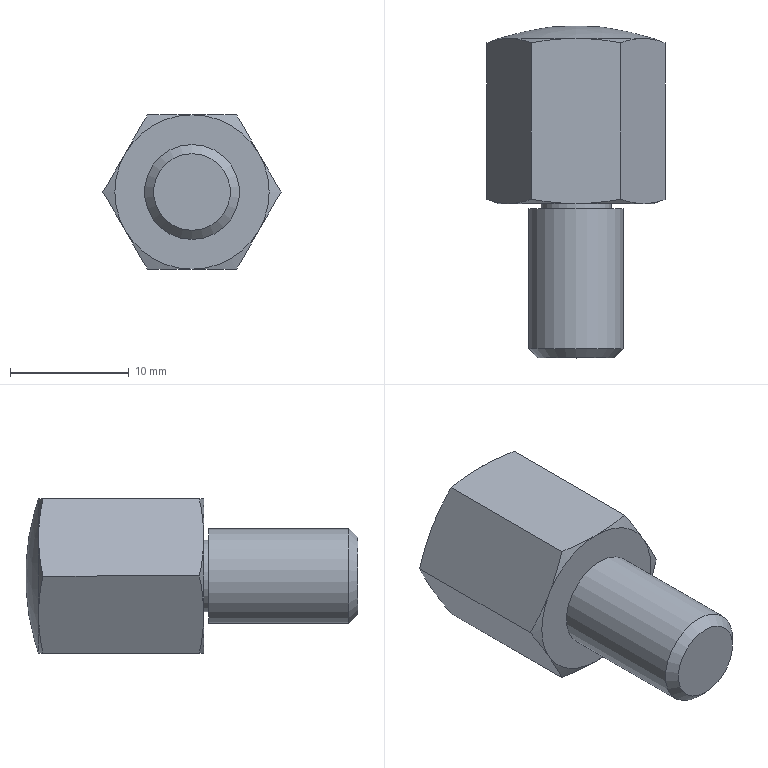Part | NX | features BREP 1 | 1 solid | 25 faces | box 15.011 x 28 x 13 mm | volume 2743 mm3 | cone 13 | plane 9 | cylinder 2 | sphere 1 | commonest cylinder face diameters 6 x1 8 x1
STEP:
#1=CARTESIAN_POINT('',(0.,-0.4333,4.));
#2=VERTEX_POINT('',#1);
#3=CARTESIAN_POINT('',(0.,-0.4333,0.));
#4=DIRECTION('',(0.,-1.,0.));
#5=DIRECTION('',(0.,0.,1.));
#6=AXIS2_PLACEMENT_3D('',#3,#4,#5);
#7=CIRCLE('',#6,4.);
#8=EDGE_CURVE('',#2,#2,#7,.T.);
#9=ORIENTED_EDGE('',*,*,#8,.T.);
#10=EDGE_LOOP('',(#9));
#11=FACE_BOUND('',#10,.T.);
#12=CARTESIAN_POINT('',(0.,-12.233,4.));
#13=VERTEX_POINT('',#12);
#14=CARTESIAN_POINT('',(0.,-12.233,0.));
#15=DIRECTION('',(0.,1.,0.));
#16=DIRECTION('',(0.,0.,1.));
#17=AXIS2_PLACEMENT_3D('',#14,#15,#16);
#18=CIRCLE('',#17,4.);
#19=EDGE_CURVE('',#13,#13,#18,.T.);
#20=ORIENTED_EDGE('',*,*,#19,.T.);
#21=EDGE_LOOP('',(#20));
#22=FACE_BOUND('',#21,.T.);
#23=CARTESIAN_POINT('',(0.,-6.333,0.));
#24=DIRECTION('',(0.,1.,0.));
#25=DIRECTION('',(0.,0.,-1.));
#26=AXIS2_PLACEMENT_3D('',#23,#24,#25);
#27=CYLINDRICAL_SURFACE('',#26,4.);
#28=ADVANCED_FACE('',(#11,#22),#27,.T.);
#29=ORIENTED_EDGE('',*,*,#8,.F.);
#30=EDGE_LOOP('',(#29));
#31=FACE_BOUND('',#30,.T.);
#32=CARTESIAN_POINT('',(0.,-0.4333,3.));
#33=VERTEX_POINT('',#32);
#34=CARTESIAN_POINT('',(0.,-0.4333,0.));
#35=DIRECTION('',(0.,-1.,0.));
#36=DIRECTION('',(0.,0.,1.));
#37=AXIS2_PLACEMENT_3D('',#34,#35,#36);
#38=CIRCLE('',#37,3.);
#39=EDGE_CURVE('',#33,#33,#38,.T.);
#40=ORIENTED_EDGE('',*,*,#39,.T.);
#41=EDGE_LOOP('',(#40));
#42=FACE_BOUND('',#41,.T.);
#43=CARTESIAN_POINT('',(3.5,-0.4333,0.));
#44=DIRECTION('',(0.,1.,0.));
#45=DIRECTION('',(0.,0.,-1.));
#46=AXIS2_PLACEMENT_3D('',#43,#44,#45);
#47=PLANE('',#46);
#48=ADVANCED_FACE('',(#31,#42),#47,.T.);
#49=ORIENTED_EDGE('',*,*,#19,.F.);
#50=EDGE_LOOP('',(#49));
#51=FACE_BOUND('',#50,.T.);
#52=CARTESIAN_POINT('',(0.,-13.,3.233));
#53=VERTEX_POINT('',#52);
#54=CARTESIAN_POINT('',(0.,-13.,0.));
#55=DIRECTION('',(0.,1.,0.));
#56=DIRECTION('',(0.,0.,1.));
#57=AXIS2_PLACEMENT_3D('',#54,#55,#56);
#58=CIRCLE('',#57,3.233);
#59=EDGE_CURVE('',#53,#53,#58,.T.);
#60=ORIENTED_EDGE('',*,*,#59,.T.);
#61=EDGE_LOOP('',(#60));
#62=FACE_BOUND('',#61,.T.);
#63=CARTESIAN_POINT('',(0.,-12.233,0.));
#64=DIRECTION('',(0.,1.,0.));
#65=DIRECTION('',(0.,0.,-1.));
#66=AXIS2_PLACEMENT_3D('',#63,#64,#65);
#67=CONICAL_SURFACE('',#66,4.,0.7854);
#68=ADVANCED_FACE('',(#51,#62),#67,.T.);
#69=ORIENTED_EDGE('',*,*,#39,.F.);
#70=EDGE_LOOP('',(#69));
#71=FACE_BOUND('',#70,.T.);
#72=CARTESIAN_POINT('',(0.,0.,3.));
#73=VERTEX_POINT('',#72);
#74=CARTESIAN_POINT('',(0.,0.,0.));
#75=DIRECTION('',(0.,-1.,0.));
#76=DIRECTION('',(0.,0.,1.));
#77=AXIS2_PLACEMENT_3D('',#74,#75,#76);
#78=CIRCLE('',#77,3.);
#79=EDGE_CURVE('',#73,#73,#78,.T.);
#80=ORIENTED_EDGE('',*,*,#79,.T.);
#81=EDGE_LOOP('',(#80));
#82=FACE_BOUND('',#81,.T.);
#83=CARTESIAN_POINT('',(0.,-0.2167,0.));
#84=DIRECTION('',(0.,1.,0.));
#85=DIRECTION('',(0.,0.,-1.));
#86=AXIS2_PLACEMENT_3D('',#83,#84,#85);
#87=CYLINDRICAL_SURFACE('',#86,3.);
#88=ADVANCED_FACE('',(#71,#82),#87,.T.);
#89=ORIENTED_EDGE('',*,*,#59,.F.);
#90=EDGE_LOOP('',(#89));
#91=FACE_BOUND('',#90,.T.);
#92=CARTESIAN_POINT('',(1.617,-13.,0.));
#93=DIRECTION('',(0.,-1.,0.));
#94=DIRECTION('',(0.,0.,1.));
#95=AXIS2_PLACEMENT_3D('',#92,#93,#94);
#96=PLANE('',#95);
#97=ADVANCED_FACE('',(#91),#96,.T.);
#98=CARTESIAN_POINT('',(0.,0.,-6.5));
#99=VERTEX_POINT('',#98);
#100=CARTESIAN_POINT('',(5.629,0.,-3.25));
#101=VERTEX_POINT('',#100);
#102=CARTESIAN_POINT('',(0.,0.,0.));
#103=DIRECTION('',(0.,-1.,0.));
#104=DIRECTION('',(0.,0.,1.));
#105=AXIS2_PLACEMENT_3D('',#102,#103,#104);
#106=CIRCLE('',#105,6.5);
#107=EDGE_CURVE('',#99,#101,#106,.T.);
#108=ORIENTED_EDGE('',*,*,#107,.T.);
#109=CARTESIAN_POINT('',(5.629,0.,3.25));
#110=VERTEX_POINT('',#109);
#111=CARTESIAN_POINT('',(0.,0.,0.));
#112=DIRECTION('',(0.,-1.,0.));
#113=DIRECTION('',(0.,0.,1.));
#114=AXIS2_PLACEMENT_3D('',#111,#112,#113);
#115=CIRCLE('',#114,6.5);
#116=EDGE_CURVE('',#101,#110,#115,.T.);
#117=ORIENTED_EDGE('',*,*,#116,.T.);
#118=CARTESIAN_POINT('',(0.,0.,6.5));
#119=VERTEX_POINT('',#118);
#120=CARTESIAN_POINT('',(0.,0.,0.));
#121=DIRECTION('',(0.,-1.,0.));
#122=DIRECTION('',(0.,0.,1.));
#123=AXIS2_PLACEMENT_3D('',#120,#121,#122);
#124=CIRCLE('',#123,6.5);
#125=EDGE_CURVE('',#110,#119,#124,.T.);
#126=ORIENTED_EDGE('',*,*,#125,.T.);
#127=CARTESIAN_POINT('',(-5.629,0.,3.25));
#128=VERTEX_POINT('',#127);
#129=CARTESIAN_POINT('',(0.,0.,0.));
#130=DIRECTION('',(0.,-1.,0.));
#131=DIRECTION('',(0.,0.,1.));
#132=AXIS2_PLACEMENT_3D('',#129,#130,#131);
#133=CIRCLE('',#132,6.5);
#134=EDGE_CURVE('',#119,#128,#133,.T.);
#135=ORIENTED_EDGE('',*,*,#134,.T.);
#136=CARTESIAN_POINT('',(-5.629,0.,-3.25));
#137=VERTEX_POINT('',#136);
#138=CARTESIAN_POINT('',(0.,0.,0.));
#139=DIRECTION('',(0.,-1.,0.));
#140=DIRECTION('',(0.,0.,1.));
#141=AXIS2_PLACEMENT_3D('',#138,#139,#140);
#142=CIRCLE('',#141,6.5);
#143=EDGE_CURVE('',#128,#137,#142,.T.);
#144=ORIENTED_EDGE('',*,*,#143,.T.);
#145=CARTESIAN_POINT('',(0.,0.,0.));
#146=DIRECTION('',(0.,-1.,0.));
#147=DIRECTION('',(0.,0.,1.));
#148=AXIS2_PLACEMENT_3D('',#145,#146,#147);
#149=CIRCLE('',#148,6.5);
#150=EDGE_CURVE('',#137,#99,#149,.T.);
#151=ORIENTED_EDGE('',*,*,#150,.T.);
#152=EDGE_LOOP('',(#108,#117,#126,#135,#144,#151));
#153=FACE_BOUND('',#152,.T.);
#154=ORIENTED_EDGE('',*,*,#79,.F.);
#155=EDGE_LOOP('',(#154));
#156=FACE_BOUND('',#155,.T.);
#157=CARTESIAN_POINT('',(4.75,0.,0.));
#158=DIRECTION('',(0.,-1.,0.));
#159=DIRECTION('',(0.,0.,1.));
#160=AXIS2_PLACEMENT_3D('',#157,#158,#159);
#161=PLANE('',#160);
#162=ADVANCED_FACE('',(#153,#156),#161,.T.);
#163=ORIENTED_EDGE('',*,*,#116,.F.);
#164=CARTESIAN_POINT('',(7.506,0.366,0.));
#165=VERTEX_POINT('',#164);
#166=CARTESIAN_POINT('',(5.629,0.,-3.25));
#167=CARTESIAN_POINT('',(6.261,0.,-2.156));
#168=CARTESIAN_POINT('',(6.885,0.1402,-1.075));
#169=CARTESIAN_POINT('',(7.506,0.366,0.));
#170=B_SPLINE_CURVE_WITH_KNOTS('',3,(#166,#167,#168,#169),.UNSPECIFIED.,.F.,.F.,(4,4),(0.,0.003771),.UNSPECIFIED.);
#171=EDGE_CURVE('',#101,#165,#170,.T.);
#172=ORIENTED_EDGE('',*,*,#171,.T.);
#173=CARTESIAN_POINT('',(7.506,0.366,0.));
#174=CARTESIAN_POINT('',(6.885,0.1402,1.075));
#175=CARTESIAN_POINT('',(6.261,0.,2.156));
#176=CARTESIAN_POINT('',(5.629,0.,3.25));
#177=B_SPLINE_CURVE_WITH_KNOTS('',3,(#173,#174,#175,#176),.UNSPECIFIED.,.F.,.F.,(4,4),(0.,0.003771),.UNSPECIFIED.);
#178=EDGE_CURVE('',#165,#110,#177,.T.);
#179=ORIENTED_EDGE('',*,*,#178,.T.);
#180=EDGE_LOOP('',(#163,#172,#179));
#181=FACE_BOUND('',#180,.T.);
#182=CARTESIAN_POINT('',(0.,0.3682,0.));
#183=DIRECTION('',(0.,1.,0.));
#184=DIRECTION('',(0.,0.,-1.));
#185=AXIS2_PLACEMENT_3D('',#182,#183,#184);
#186=CONICAL_SURFACE('',#185,7.512,1.222);
#187=ADVANCED_FACE('',(#181),#186,.T.);
#188=ORIENTED_EDGE('',*,*,#107,.F.);
#189=CARTESIAN_POINT('',(3.753,0.366,-6.5));
#190=VERTEX_POINT('',#189);
#191=CARTESIAN_POINT('',(0.,0.,-6.5));
#192=CARTESIAN_POINT('',(1.263,0.,-6.5));
#193=CARTESIAN_POINT('',(2.512,0.1402,-6.5));
#194=CARTESIAN_POINT('',(3.753,0.366,-6.5));
#195=B_SPLINE_CURVE_WITH_KNOTS('',3,(#191,#192,#193,#194),.UNSPECIFIED.,.F.,.F.,(4,4),(0.,0.003771),.UNSPECIFIED.);
#196=EDGE_CURVE('',#99,#190,#195,.T.);
#197=ORIENTED_EDGE('',*,*,#196,.T.);
#198=CARTESIAN_POINT('',(3.753,0.366,-6.5));
#199=CARTESIAN_POINT('',(4.373,0.1402,-5.425));
#200=CARTESIAN_POINT('',(4.998,0.,-4.344));
#201=CARTESIAN_POINT('',(5.629,0.,-3.25));
#202=B_SPLINE_CURVE_WITH_KNOTS('',3,(#198,#199,#200,#201),.UNSPECIFIED.,.F.,.F.,(4,4),(0.,0.003771),.UNSPECIFIED.);
#203=EDGE_CURVE('',#190,#101,#202,.T.);
#204=ORIENTED_EDGE('',*,*,#203,.T.);
#205=EDGE_LOOP('',(#188,#197,#204));
#206=FACE_BOUND('',#205,.T.);
#207=CARTESIAN_POINT('',(0.,0.3682,0.));
#208=DIRECTION('',(0.,1.,0.));
#209=DIRECTION('',(0.,0.,-1.));
#210=AXIS2_PLACEMENT_3D('',#207,#208,#209);
#211=CONICAL_SURFACE('',#210,7.512,1.222);
#212=ADVANCED_FACE('',(#206),#211,.T.);
#213=CARTESIAN_POINT('',(-3.753,0.366,-6.5));
#214=VERTEX_POINT('',#213);
#215=CARTESIAN_POINT('',(-3.753,0.366,-6.5));
#216=CARTESIAN_POINT('',(-2.512,0.1402,-6.5));
#217=CARTESIAN_POINT('',(-1.263,0.,-6.5));
#218=CARTESIAN_POINT('',(0.,0.,-6.5));
#219=B_SPLINE_CURVE_WITH_KNOTS('',3,(#215,#216,#217,#218),.UNSPECIFIED.,.F.,.F.,(4,4),(0.,0.003771),.UNSPECIFIED.);
#220=EDGE_CURVE('',#214,#99,#219,.T.);
#221=ORIENTED_EDGE('',*,*,#220,.T.);
#222=ORIENTED_EDGE('',*,*,#150,.F.);
#223=CARTESIAN_POINT('',(-5.629,0.,-3.25));
#224=CARTESIAN_POINT('',(-4.998,0.,-4.344));
#225=CARTESIAN_POINT('',(-4.373,0.1402,-5.425));
#226=CARTESIAN_POINT('',(-3.753,0.366,-6.5));
#227=B_SPLINE_CURVE_WITH_KNOTS('',3,(#223,#224,#225,#226),.UNSPECIFIED.,.F.,.F.,(4,4),(0.,0.003771),.UNSPECIFIED.);
#228=EDGE_CURVE('',#137,#214,#227,.T.);
#229=ORIENTED_EDGE('',*,*,#228,.T.);
#230=EDGE_LOOP('',(#221,#222,#229));
#231=FACE_BOUND('',#230,.T.);
#232=CARTESIAN_POINT('',(0.,0.3682,0.));
#233=DIRECTION('',(0.,1.,0.));
#234=DIRECTION('',(0.,0.,-1.));
#235=AXIS2_PLACEMENT_3D('',#232,#233,#234);
#236=CONICAL_SURFACE('',#235,7.512,1.222);
#237=ADVANCED_FACE('',(#231),#236,.T.);
#238=CARTESIAN_POINT('',(-7.506,0.366,0.000000027));
#239=VERTEX_POINT('',#238);
#240=CARTESIAN_POINT('',(-5.629,0.,3.25));
#241=CARTESIAN_POINT('',(-6.261,0.,2.156));
#242=CARTESIAN_POINT('',(-6.885,0.1402,1.075));
#243=CARTESIAN_POINT('',(-7.506,0.366,0.000000017));
#244=B_SPLINE_CURVE_WITH_KNOTS('',3,(#240,#241,#242,#243),.UNSPECIFIED.,.F.,.F.,(4,4),(0.,0.003771),.UNSPECIFIED.);
#245=EDGE_CURVE('',#128,#239,#244,.T.);
#246=ORIENTED_EDGE('',*,*,#245,.T.);
#247=CARTESIAN_POINT('',(-7.506,0.366,0.000000037));
#248=CARTESIAN_POINT('',(-6.885,0.1402,-1.075));
#249=CARTESIAN_POINT('',(-6.261,0.,-2.156));
#250=CARTESIAN_POINT('',(-5.629,0.,-3.25));
#251=B_SPLINE_CURVE_WITH_KNOTS('',3,(#247,#248,#249,#250),.UNSPECIFIED.,.F.,.F.,(4,4),(0.,0.003771),.UNSPECIFIED.);
#252=EDGE_CURVE('',#239,#137,#251,.T.);
#253=ORIENTED_EDGE('',*,*,#252,.T.);
#254=ORIENTED_EDGE('',*,*,#143,.F.);
#255=EDGE_LOOP('',(#246,#253,#254));
#256=FACE_BOUND('',#255,.T.);
#257=CARTESIAN_POINT('',(0.,0.3682,0.));
#258=DIRECTION('',(0.,1.,0.));
#259=DIRECTION('',(0.,0.,-1.));
#260=AXIS2_PLACEMENT_3D('',#257,#258,#259);
#261=CONICAL_SURFACE('',#260,7.512,1.222);
#262=ADVANCED_FACE('',(#256),#261,.T.);
#263=CARTESIAN_POINT('',(-3.753,0.366,6.5));
#264=VERTEX_POINT('',#263);
#265=CARTESIAN_POINT('',(-3.753,0.366,6.5));
#266=CARTESIAN_POINT('',(-4.373,0.1402,5.425));
#267=CARTESIAN_POINT('',(-4.998,0.,4.344));
#268=CARTESIAN_POINT('',(-5.629,0.,3.25));
#269=B_SPLINE_CURVE_WITH_KNOTS('',3,(#265,#266,#267,#268),.UNSPECIFIED.,.F.,.F.,(4,4),(0.,0.003771),.UNSPECIFIED.);
#270=EDGE_CURVE('',#264,#128,#269,.T.);
#271=ORIENTED_EDGE('',*,*,#270,.T.);
#272=ORIENTED_EDGE('',*,*,#134,.F.);
#273=CARTESIAN_POINT('',(0.,0.,6.5));
#274=CARTESIAN_POINT('',(-1.263,0.,6.5));
#275=CARTESIAN_POINT('',(-2.512,0.1402,6.5));
#276=CARTESIAN_POINT('',(-3.753,0.366,6.5));
#277=B_SPLINE_CURVE_WITH_KNOTS('',3,(#273,#274,#275,#276),.UNSPECIFIED.,.F.,.F.,(4,4),(0.,0.003771),.UNSPECIFIED.);
#278=EDGE_CURVE('',#119,#264,#277,.T.);
#279=ORIENTED_EDGE('',*,*,#278,.T.);
#280=EDGE_LOOP('',(#271,#272,#279));
#281=FACE_BOUND('',#280,.T.);
#282=CARTESIAN_POINT('',(0.,0.3682,0.));
#283=DIRECTION('',(0.,1.,0.));
#284=DIRECTION('',(0.,0.,-1.));
#285=AXIS2_PLACEMENT_3D('',#282,#283,#284);
#286=CONICAL_SURFACE('',#285,7.512,1.222);
#287=ADVANCED_FACE('',(#281),#286,.T.);
#288=ORIENTED_EDGE('',*,*,#125,.F.);
#289=CARTESIAN_POINT('',(3.753,0.366,6.5));
#290=VERTEX_POINT('',#289);
#291=CARTESIAN_POINT('',(5.629,0.,3.25));
#292=CARTESIAN_POINT('',(4.998,0.,4.344));
#293=CARTESIAN_POINT('',(4.373,0.1402,5.425));
#294=CARTESIAN_POINT('',(3.753,0.366,6.5));
#295=B_SPLINE_CURVE_WITH_KNOTS('',3,(#291,#292,#293,#294),.UNSPECIFIED.,.F.,.F.,(4,4),(0.,0.003771),.UNSPECIFIED.);
#296=EDGE_CURVE('',#110,#290,#295,.T.);
#297=ORIENTED_EDGE('',*,*,#296,.T.);
#298=CARTESIAN_POINT('',(3.753,0.366,6.5));
#299=CARTESIAN_POINT('',(2.512,0.1402,6.5));
#300=CARTESIAN_POINT('',(1.263,0.,6.5));
#301=CARTESIAN_POINT('',(0.,0.,6.5));
#302=B_SPLINE_CURVE_WITH_KNOTS('',3,(#298,#299,#300,#301),.UNSPECIFIED.,.F.,.F.,(4,4),(0.,0.003771),.UNSPECIFIED.);
#303=EDGE_CURVE('',#290,#119,#302,.T.);
#304=ORIENTED_EDGE('',*,*,#303,.T.);
#305=EDGE_LOOP('',(#288,#297,#304));
#306=FACE_BOUND('',#305,.T.);
#307=CARTESIAN_POINT('',(0.,0.3682,0.));
#308=DIRECTION('',(0.,1.,0.));
#309=DIRECTION('',(0.,0.,-1.));
#310=AXIS2_PLACEMENT_3D('',#307,#308,#309);
#311=CONICAL_SURFACE('',#310,7.512,1.222);
#312=ADVANCED_FACE('',(#306),#311,.T.);
#313=ORIENTED_EDGE('',*,*,#203,.F.);
#314=CARTESIAN_POINT('',(3.753,13.548,-6.5));
#315=VERTEX_POINT('',#314);
#316=CARTESIAN_POINT('',(3.753,20.,-6.5));
#317=DIRECTION('',(0.,-1.,0.));
#318=VECTOR('',#317,1000.);
#319=LINE('',#316,#318);
#320=EDGE_CURVE('',#315,#190,#319,.T.);
#321=ORIENTED_EDGE('',*,*,#320,.F.);
#322=CARTESIAN_POINT('',(5.629,13.914,-3.25));
#323=VERTEX_POINT('',#322);
#324=CARTESIAN_POINT('',(5.629,13.914,-3.25));
#325=CARTESIAN_POINT('',(4.998,13.914,-4.344));
#326=CARTESIAN_POINT('',(4.373,13.774,-5.425));
#327=CARTESIAN_POINT('',(3.753,13.548,-6.5));
#328=B_SPLINE_CURVE_WITH_KNOTS('',3,(#324,#325,#326,#327),.UNSPECIFIED.,.F.,.F.,(4,4),(0.,0.003771),.UNSPECIFIED.);
#329=EDGE_CURVE('',#323,#315,#328,.T.);
#330=ORIENTED_EDGE('',*,*,#329,.F.);
#331=CARTESIAN_POINT('',(7.506,13.548,0.));
#332=VERTEX_POINT('',#331);
#333=CARTESIAN_POINT('',(7.506,13.548,0.));
#334=CARTESIAN_POINT('',(6.885,13.774,-1.075));
#335=CARTESIAN_POINT('',(6.261,13.914,-2.156));
#336=CARTESIAN_POINT('',(5.629,13.914,-3.25));
#337=B_SPLINE_CURVE_WITH_KNOTS('',3,(#333,#334,#335,#336),.UNSPECIFIED.,.F.,.F.,(4,4),(0.,0.003771),.UNSPECIFIED.);
#338=EDGE_CURVE('',#332,#323,#337,.T.);
#339=ORIENTED_EDGE('',*,*,#338,.F.);
#340=CARTESIAN_POINT('',(7.506,20.,0.));
#341=DIRECTION('',(0.,1.,0.));
#342=VECTOR('',#341,1000.);
#343=LINE('',#340,#342);
#344=EDGE_CURVE('',#165,#332,#343,.T.);
#345=ORIENTED_EDGE('',*,*,#344,.F.);
#346=ORIENTED_EDGE('',*,*,#171,.F.);
#347=EDGE_LOOP('',(#313,#321,#330,#339,#345,#346));
#348=FACE_BOUND('',#347,.T.);
#349=CARTESIAN_POINT('',(3.753,20.,-6.5));
#350=DIRECTION('',(-0.866,0.,0.5));
#351=DIRECTION('',(-0.5,0.,-0.866));
#352=AXIS2_PLACEMENT_3D('',#349,#350,#351);
#353=PLANE('',#352);
#354=ADVANCED_FACE('',(#348),#353,.F.);
#355=ORIENTED_EDGE('',*,*,#220,.F.);
#356=CARTESIAN_POINT('',(-3.753,13.548,-6.5));
#357=VERTEX_POINT('',#356);
#358=CARTESIAN_POINT('',(-3.753,20.,-6.5));
#359=DIRECTION('',(0.,-1.,0.));
#360=VECTOR('',#359,1000.);
#361=LINE('',#358,#360);
#362=EDGE_CURVE('',#357,#214,#361,.T.);
#363=ORIENTED_EDGE('',*,*,#362,.F.);
#364=CARTESIAN_POINT('',(0.,13.914,-6.5));
#365=VERTEX_POINT('',#364);
#366=CARTESIAN_POINT('',(0.,13.914,-6.5));
#367=CARTESIAN_POINT('',(-1.263,13.914,-6.5));
#368=CARTESIAN_POINT('',(-2.512,13.774,-6.5));
#369=CARTESIAN_POINT('',(-3.753,13.548,-6.5));
#370=B_SPLINE_CURVE_WITH_KNOTS('',3,(#366,#367,#368,#369),.UNSPECIFIED.,.F.,.F.,(4,4),(0.,0.003771),.UNSPECIFIED.);
#371=EDGE_CURVE('',#365,#357,#370,.T.);
#372=ORIENTED_EDGE('',*,*,#371,.F.);
#373=CARTESIAN_POINT('',(3.753,13.548,-6.5));
#374=CARTESIAN_POINT('',(2.512,13.774,-6.5));
#375=CARTESIAN_POINT('',(1.263,13.914,-6.5));
#376=CARTESIAN_POINT('',(0.,13.914,-6.5));
#377=B_SPLINE_CURVE_WITH_KNOTS('',3,(#373,#374,#375,#376),.UNSPECIFIED.,.F.,.F.,(4,4),(0.,0.003771),.UNSPECIFIED.);
#378=EDGE_CURVE('',#315,#365,#377,.T.);
#379=ORIENTED_EDGE('',*,*,#378,.F.);
#380=ORIENTED_EDGE('',*,*,#320,.T.);
#381=ORIENTED_EDGE('',*,*,#196,.F.);
#382=EDGE_LOOP('',(#355,#363,#372,#379,#380,#381));
#383=FACE_BOUND('',#382,.T.);
#384=CARTESIAN_POINT('',(-3.753,20.,-6.5));
#385=DIRECTION('',(0.,0.,1.));
#386=DIRECTION('',(-1.,0.,0.));
#387=AXIS2_PLACEMENT_3D('',#384,#385,#386);
#388=PLANE('',#387);
#389=ADVANCED_FACE('',(#383),#388,.F.);
#390=CARTESIAN_POINT('',(-7.506,13.548,0.));
#391=VERTEX_POINT('',#390);
#392=CARTESIAN_POINT('',(-7.506,20.,0.));
#393=DIRECTION('',(0.,-1.,0.));
#394=VECTOR('',#393,1000.);
#395=LINE('',#392,#394);
#396=EDGE_CURVE('',#391,#239,#395,.T.);
#397=ORIENTED_EDGE('',*,*,#396,.F.);
#398=CARTESIAN_POINT('',(-5.629,13.914,-3.25));
#399=VERTEX_POINT('',#398);
#400=CARTESIAN_POINT('',(-5.629,13.914,-3.25));
#401=CARTESIAN_POINT('',(-6.261,13.914,-2.156));
#402=CARTESIAN_POINT('',(-6.885,13.774,-1.075));
#403=CARTESIAN_POINT('',(-7.506,13.548,0.));
#404=B_SPLINE_CURVE_WITH_KNOTS('',3,(#400,#401,#402,#403),.UNSPECIFIED.,.F.,.F.,(4,4),(0.,0.003771),.UNSPECIFIED.);
#405=EDGE_CURVE('',#399,#391,#404,.T.);
#406=ORIENTED_EDGE('',*,*,#405,.F.);
#407=CARTESIAN_POINT('',(-3.753,13.548,-6.5));
#408=CARTESIAN_POINT('',(-4.373,13.774,-5.425));
#409=CARTESIAN_POINT('',(-4.998,13.914,-4.344));
#410=CARTESIAN_POINT('',(-5.629,13.914,-3.25));
#411=B_SPLINE_CURVE_WITH_KNOTS('',3,(#407,#408,#409,#410),.UNSPECIFIED.,.F.,.F.,(4,4),(0.,0.003771),.UNSPECIFIED.);
#412=EDGE_CURVE('',#357,#399,#411,.T.);
#413=ORIENTED_EDGE('',*,*,#412,.F.);
#414=ORIENTED_EDGE('',*,*,#362,.T.);
#415=ORIENTED_EDGE('',*,*,#228,.F.);
#416=ORIENTED_EDGE('',*,*,#252,.F.);
#417=EDGE_LOOP('',(#397,#406,#413,#414,#415,#416));
#418=FACE_BOUND('',#417,.T.);
#419=CARTESIAN_POINT('',(-7.506,20.,0.));
#420=DIRECTION('',(0.866,0.,0.5));
#421=DIRECTION('',(-0.5,0.,0.866));
#422=AXIS2_PLACEMENT_3D('',#419,#420,#421);
#423=PLANE('',#422);
#424=ADVANCED_FACE('',(#418),#423,.F.);
#425=CARTESIAN_POINT('',(-3.753,13.548,6.5));
#426=VERTEX_POINT('',#425);
#427=CARTESIAN_POINT('',(-3.753,20.,6.5));
#428=DIRECTION('',(0.,-1.,0.));
#429=VECTOR('',#428,1000.);
#430=LINE('',#427,#429);
#431=EDGE_CURVE('',#426,#264,#430,.T.);
#432=ORIENTED_EDGE('',*,*,#431,.F.);
#433=CARTESIAN_POINT('',(-5.629,13.914,3.25));
#434=VERTEX_POINT('',#433);
#435=CARTESIAN_POINT('',(-5.629,13.914,3.25));
#436=CARTESIAN_POINT('',(-4.998,13.914,4.344));
#437=CARTESIAN_POINT('',(-4.373,13.774,5.425));
#438=CARTESIAN_POINT('',(-3.753,13.548,6.5));
#439=B_SPLINE_CURVE_WITH_KNOTS('',3,(#435,#436,#437,#438),.UNSPECIFIED.,.F.,.F.,(4,4),(0.,0.003771),.UNSPECIFIED.);
#440=EDGE_CURVE('',#434,#426,#439,.T.);
#441=ORIENTED_EDGE('',*,*,#440,.F.);
#442=CARTESIAN_POINT('',(-7.506,13.548,0.));
#443=CARTESIAN_POINT('',(-6.885,13.774,1.075));
#444=CARTESIAN_POINT('',(-6.261,13.914,2.156));
#445=CARTESIAN_POINT('',(-5.629,13.914,3.25));
#446=B_SPLINE_CURVE_WITH_KNOTS('',3,(#442,#443,#444,#445),.UNSPECIFIED.,.F.,.F.,(4,4),(0.,0.003771),.UNSPECIFIED.);
#447=EDGE_CURVE('',#391,#434,#446,.T.);
#448=ORIENTED_EDGE('',*,*,#447,.F.);
#449=ORIENTED_EDGE('',*,*,#396,.T.);
#450=ORIENTED_EDGE('',*,*,#245,.F.);
#451=ORIENTED_EDGE('',*,*,#270,.F.);
#452=EDGE_LOOP('',(#432,#441,#448,#449,#450,#451));
#453=FACE_BOUND('',#452,.T.);
#454=CARTESIAN_POINT('',(-3.753,20.,6.5));
#455=DIRECTION('',(0.866,0.,-0.5));
#456=DIRECTION('',(0.5,0.,0.866));
#457=AXIS2_PLACEMENT_3D('',#454,#455,#456);
#458=PLANE('',#457);
#459=ADVANCED_FACE('',(#453),#458,.F.);
#460=CARTESIAN_POINT('',(3.753,13.548,6.5));
#461=VERTEX_POINT('',#460);
#462=CARTESIAN_POINT('',(3.753,20.,6.5));
#463=DIRECTION('',(0.,-1.,0.));
#464=VECTOR('',#463,1000.);
#465=LINE('',#462,#464);
#466=EDGE_CURVE('',#461,#290,#465,.T.);
#467=ORIENTED_EDGE('',*,*,#466,.F.);
#468=CARTESIAN_POINT('',(0.,13.914,6.5));
#469=VERTEX_POINT('',#468);
#470=CARTESIAN_POINT('',(0.,13.914,6.5));
#471=CARTESIAN_POINT('',(1.263,13.914,6.5));
#472=CARTESIAN_POINT('',(2.512,13.774,6.5));
#473=CARTESIAN_POINT('',(3.753,13.548,6.5));
#474=B_SPLINE_CURVE_WITH_KNOTS('',3,(#470,#471,#472,#473),.UNSPECIFIED.,.F.,.F.,(4,4),(0.,0.003771),.UNSPECIFIED.);
#475=EDGE_CURVE('',#469,#461,#474,.T.);
#476=ORIENTED_EDGE('',*,*,#475,.F.);
#477=CARTESIAN_POINT('',(-3.753,13.548,6.5));
#478=CARTESIAN_POINT('',(-2.512,13.774,6.5));
#479=CARTESIAN_POINT('',(-1.263,13.914,6.5));
#480=CARTESIAN_POINT('',(0.,13.914,6.5));
#481=B_SPLINE_CURVE_WITH_KNOTS('',3,(#477,#478,#479,#480),.UNSPECIFIED.,.F.,.F.,(4,4),(0.,0.003771),.UNSPECIFIED.);
#482=EDGE_CURVE('',#426,#469,#481,.T.);
#483=ORIENTED_EDGE('',*,*,#482,.F.);
#484=ORIENTED_EDGE('',*,*,#431,.T.);
#485=ORIENTED_EDGE('',*,*,#278,.F.);
#486=ORIENTED_EDGE('',*,*,#303,.F.);
#487=EDGE_LOOP('',(#467,#476,#483,#484,#485,#486));
#488=FACE_BOUND('',#487,.T.);
#489=CARTESIAN_POINT('',(3.753,20.,6.5));
#490=DIRECTION('',(0.,0.,-1.));
#491=DIRECTION('',(1.,0.,0.));
#492=AXIS2_PLACEMENT_3D('',#489,#490,#491);
#493=PLANE('',#492);
#494=ADVANCED_FACE('',(#488),#493,.F.);
#495=ORIENTED_EDGE('',*,*,#178,.F.);
#496=ORIENTED_EDGE('',*,*,#344,.T.);
#497=CARTESIAN_POINT('',(5.629,13.914,3.25));
#498=VERTEX_POINT('',#497);
#499=CARTESIAN_POINT('',(5.629,13.914,3.25));
#500=CARTESIAN_POINT('',(6.261,13.914,2.156));
#501=CARTESIAN_POINT('',(6.885,13.774,1.075));
#502=CARTESIAN_POINT('',(7.506,13.548,0.));
#503=B_SPLINE_CURVE_WITH_KNOTS('',3,(#499,#500,#501,#502),.UNSPECIFIED.,.F.,.F.,(4,4),(0.,0.003771),.UNSPECIFIED.);
#504=EDGE_CURVE('',#498,#332,#503,.T.);
#505=ORIENTED_EDGE('',*,*,#504,.F.);
#506=CARTESIAN_POINT('',(3.753,13.548,6.5));
#507=CARTESIAN_POINT('',(4.373,13.774,5.425));
#508=CARTESIAN_POINT('',(4.998,13.914,4.344));
#509=CARTESIAN_POINT('',(5.629,13.914,3.25));
#510=B_SPLINE_CURVE_WITH_KNOTS('',3,(#506,#507,#508,#509),.UNSPECIFIED.,.F.,.F.,(4,4),(0.,0.003771),.UNSPECIFIED.);
#511=EDGE_CURVE('',#461,#498,#510,.T.);
#512=ORIENTED_EDGE('',*,*,#511,.F.);
#513=ORIENTED_EDGE('',*,*,#466,.T.);
#514=ORIENTED_EDGE('',*,*,#296,.F.);
#515=EDGE_LOOP('',(#495,#496,#505,#512,#513,#514));
#516=FACE_BOUND('',#515,.T.);
#517=CARTESIAN_POINT('',(7.506,20.,0.));
#518=DIRECTION('',(-0.866,0.,-0.5));
#519=DIRECTION('',(0.5,0.,-0.866));
#520=AXIS2_PLACEMENT_3D('',#517,#518,#519);
#521=PLANE('',#520);
#522=ADVANCED_FACE('',(#516),#521,.F.);
#523=ORIENTED_EDGE('',*,*,#378,.T.);
#524=CARTESIAN_POINT('',(0.,13.914,0.));
#525=DIRECTION('',(0.,-1.,0.));
#526=DIRECTION('',(0.,0.,-1.));
#527=AXIS2_PLACEMENT_3D('',#524,#525,#526);
#528=CIRCLE('',#527,6.5);
#529=EDGE_CURVE('',#365,#323,#528,.T.);
#530=ORIENTED_EDGE('',*,*,#529,.T.);
#531=ORIENTED_EDGE('',*,*,#329,.T.);
#532=EDGE_LOOP('',(#523,#530,#531));
#533=FACE_BOUND('',#532,.T.);
#534=CARTESIAN_POINT('',(0.,13.546,0.));
#535=DIRECTION('',(0.,-1.,0.));
#536=DIRECTION('',(0.,0.,1.));
#537=AXIS2_PLACEMENT_3D('',#534,#535,#536);
#538=CONICAL_SURFACE('',#537,7.512,1.222);
#539=ADVANCED_FACE('',(#533),#538,.T.);
#540=CARTESIAN_POINT('',(0.,13.914,0.));
#541=DIRECTION('',(0.,-1.,0.));
#542=DIRECTION('',(0.,0.,-1.));
#543=AXIS2_PLACEMENT_3D('',#540,#541,#542);
#544=CIRCLE('',#543,6.5);
#545=EDGE_CURVE('',#323,#498,#544,.T.);
#546=ORIENTED_EDGE('',*,*,#545,.T.);
#547=ORIENTED_EDGE('',*,*,#504,.T.);
#548=ORIENTED_EDGE('',*,*,#338,.T.);
#549=EDGE_LOOP('',(#546,#547,#548));
#550=FACE_BOUND('',#549,.T.);
#551=CARTESIAN_POINT('',(0.,13.546,0.));
#552=DIRECTION('',(0.,-1.,0.));
#553=DIRECTION('',(0.,0.,1.));
#554=AXIS2_PLACEMENT_3D('',#551,#552,#553);
#555=CONICAL_SURFACE('',#554,7.512,1.222);
#556=ADVANCED_FACE('',(#550),#555,.T.);
#557=ORIENTED_EDGE('',*,*,#412,.T.);
#558=CARTESIAN_POINT('',(0.,13.914,0.));
#559=DIRECTION('',(0.,-1.,0.));
#560=DIRECTION('',(0.,0.,-1.));
#561=AXIS2_PLACEMENT_3D('',#558,#559,#560);
#562=CIRCLE('',#561,6.5);
#563=EDGE_CURVE('',#399,#365,#562,.T.);
#564=ORIENTED_EDGE('',*,*,#563,.T.);
#565=ORIENTED_EDGE('',*,*,#371,.T.);
#566=EDGE_LOOP('',(#557,#564,#565));
#567=FACE_BOUND('',#566,.T.);
#568=CARTESIAN_POINT('',(0.,13.546,0.));
#569=DIRECTION('',(0.,-1.,0.));
#570=DIRECTION('',(0.,0.,1.));
#571=AXIS2_PLACEMENT_3D('',#568,#569,#570);
#572=CONICAL_SURFACE('',#571,7.512,1.222);
#573=ADVANCED_FACE('',(#567),#572,.T.);
#574=ORIENTED_EDGE('',*,*,#447,.T.);
#575=CARTESIAN_POINT('',(0.,13.914,0.));
#576=DIRECTION('',(0.,-1.,0.));
#577=DIRECTION('',(0.,0.,-1.));
#578=AXIS2_PLACEMENT_3D('',#575,#576,#577);
#579=CIRCLE('',#578,6.5);
#580=EDGE_CURVE('',#434,#399,#579,.T.);
#581=ORIENTED_EDGE('',*,*,#580,.T.);
#582=ORIENTED_EDGE('',*,*,#405,.T.);
#583=EDGE_LOOP('',(#574,#581,#582));
#584=FACE_BOUND('',#583,.T.);
#585=CARTESIAN_POINT('',(0.,13.546,0.));
#586=DIRECTION('',(0.,-1.,0.));
#587=DIRECTION('',(0.,0.,1.));
#588=AXIS2_PLACEMENT_3D('',#585,#586,#587);
#589=CONICAL_SURFACE('',#588,7.512,1.222);
#590=ADVANCED_FACE('',(#584),#589,.T.);
#591=CARTESIAN_POINT('',(0.,13.914,0.));
#592=DIRECTION('',(0.,-1.,0.));
#593=DIRECTION('',(0.,0.,-1.));
#594=AXIS2_PLACEMENT_3D('',#591,#592,#593);
#595=CIRCLE('',#594,6.5);
#596=EDGE_CURVE('',#469,#434,#595,.T.);
#597=ORIENTED_EDGE('',*,*,#596,.T.);
#598=ORIENTED_EDGE('',*,*,#440,.T.);
#599=ORIENTED_EDGE('',*,*,#482,.T.);
#600=EDGE_LOOP('',(#597,#598,#599));
#601=FACE_BOUND('',#600,.T.);
#602=CARTESIAN_POINT('',(0.,13.546,0.));
#603=DIRECTION('',(0.,-1.,0.));
#604=DIRECTION('',(0.,0.,1.));
#605=AXIS2_PLACEMENT_3D('',#602,#603,#604);
#606=CONICAL_SURFACE('',#605,7.512,1.222);
#607=ADVANCED_FACE('',(#601),#606,.T.);
#608=CARTESIAN_POINT('',(0.,13.914,0.));
#609=DIRECTION('',(0.,-1.,0.));
#610=DIRECTION('',(0.,0.,-1.));
#611=AXIS2_PLACEMENT_3D('',#608,#609,#610);
#612=CIRCLE('',#611,6.5);
#613=EDGE_CURVE('',#498,#469,#612,.T.);
#614=ORIENTED_EDGE('',*,*,#613,.T.);
#615=ORIENTED_EDGE('',*,*,#475,.T.);
#616=ORIENTED_EDGE('',*,*,#511,.T.);
#617=EDGE_LOOP('',(#614,#615,#616));
#618=FACE_BOUND('',#617,.T.);
#619=CARTESIAN_POINT('',(0.,13.546,0.));
#620=DIRECTION('',(0.,-1.,0.));
#621=DIRECTION('',(0.,0.,1.));
#622=AXIS2_PLACEMENT_3D('',#619,#620,#621);
#623=CONICAL_SURFACE('',#622,7.512,1.222);
#624=ADVANCED_FACE('',(#618),#623,.T.);
#625=ORIENTED_EDGE('',*,*,#596,.F.);
#626=ORIENTED_EDGE('',*,*,#613,.F.);
#627=ORIENTED_EDGE('',*,*,#545,.F.);
#628=ORIENTED_EDGE('',*,*,#529,.F.);
#629=ORIENTED_EDGE('',*,*,#563,.F.);
#630=ORIENTED_EDGE('',*,*,#580,.F.);
#631=EDGE_LOOP('',(#625,#626,#627,#628,#629,#630));
#632=FACE_BOUND('',#631,.T.);
#633=CARTESIAN_POINT('',(0.,-5.,0.));
#634=DIRECTION('',(1.,0.,0.));
#635=DIRECTION('',(0.,0.9444,-0.3288));
#636=AXIS2_PLACEMENT_3D('',#633,#634,#635);
#637=SPHERICAL_SURFACE('',#636,20.);
#638=ADVANCED_FACE('',(#632),#637,.T.);
#639=CLOSED_SHELL('',(#28,#48,#68,#88,#97,#162,#187,#212,#237,#262,#287,#312,#354,#389,#424,#459,#494,#522,#539,#556,#573,#590,#607,#624,#638));
#640=MANIFOLD_SOLID_BREP('',#639);
#641=(LENGTH_UNIT()NAMED_UNIT(*)SI_UNIT(.MILLI.,.METRE.));
#642=UNCERTAINTY_MEASURE_WITH_UNIT(LENGTH_MEASURE(0.0508),#641,'','');
#643=(NAMED_UNIT(*)PLANE_ANGLE_UNIT()SI_UNIT($,.RADIAN.));
#644=(NAMED_UNIT(*)SI_UNIT($,.STERADIAN.)SOLID_ANGLE_UNIT());
#645=(GEOMETRIC_REPRESENTATION_CONTEXT(3)GLOBAL_UNCERTAINTY_ASSIGNED_CONTEXT((#642))GLOBAL_UNIT_ASSIGNED_CONTEXT((#641,#643,#644))REPRESENTATION_CONTEXT('',''));
#646=ADVANCED_BREP_SHAPE_REPRESENTATION('',(#640),#645);